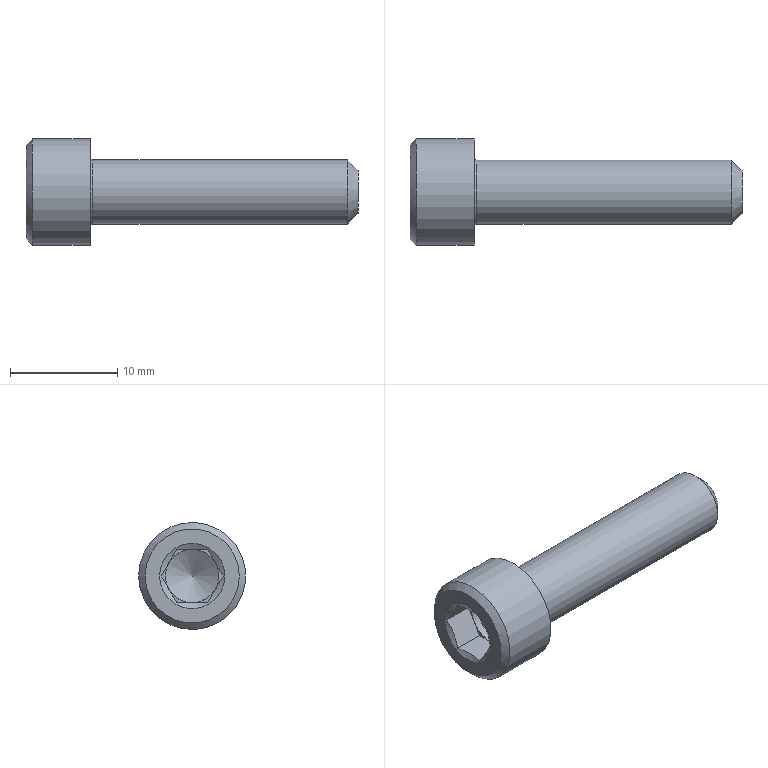Part | STEP file | Винт М6-6gx25 ГОСТ 11738-84 | 1 solid | 23 faces | box 31 x 10 x 10 mm | volume 1075 mm3 | plane 15 | cone 4 | cylinder 3 | torus 1 | commonest cylinder face diameters 5 x1 6 x1 10 x1
STEP:
#1=CARTESIAN_POINT('',(-6.,4.4,0.));
#2=VERTEX_POINT('',#1);
#3=CARTESIAN_POINT('',(-6.,0.,0.));
#4=DIRECTION('',(1.,0.,0.));
#5=DIRECTION('',(0.,1.,0.));
#6=AXIS2_PLACEMENT_3D('',#3,#4,#5);
#7=CIRCLE('',#6,4.4);
#8=EDGE_CURVE('',#2,#2,#7,.T.);
#9=ORIENTED_EDGE('',*,*,#8,.F.);
#10=EDGE_LOOP('',(#9));
#11=FACE_BOUND('',#10,.T.);
#12=CARTESIAN_POINT('',(-6.,3.05,0.));
#13=VERTEX_POINT('',#12);
#14=CARTESIAN_POINT('',(-6.,0.,0.));
#15=DIRECTION('',(1.,0.,0.));
#16=DIRECTION('',(0.,1.,0.));
#17=AXIS2_PLACEMENT_3D('',#14,#15,#16);
#18=CIRCLE('',#17,3.05);
#19=EDGE_CURVE('',#13,#13,#18,.T.);
#20=ORIENTED_EDGE('',*,*,#19,.T.);
#21=EDGE_LOOP('',(#20));
#22=FACE_BOUND('',#21,.T.);
#23=CARTESIAN_POINT('',(-6.,0.,0.));
#24=DIRECTION('',(-1.,0.,0.));
#25=DIRECTION('',(0.,1.,0.));
#26=AXIS2_PLACEMENT_3D('',#23,#24,#25);
#27=PLANE('',#26);
#28=ADVANCED_FACE('',(#11,#22),#27,.T.);
#29=CARTESIAN_POINT('',(-5.906,1.443,-2.5));
#30=VERTEX_POINT('',#29);
#31=CARTESIAN_POINT('',(-5.906,-1.443,-2.5));
#32=VERTEX_POINT('',#31);
#33=CARTESIAN_POINT('',(-5.906,1.443,-2.5));
#34=CARTESIAN_POINT('',(-5.9,1.424,-2.5));
#35=CARTESIAN_POINT('',(-5.89,1.389,-2.5));
#36=CARTESIAN_POINT('',(-5.88,1.351,-2.5));
#37=CARTESIAN_POINT('',(-5.867,1.304,-2.5));
#38=CARTESIAN_POINT('',(-5.848,1.232,-2.5));
#39=CARTESIAN_POINT('',(-5.827,1.146,-2.5));
#40=CARTESIAN_POINT('',(-5.803,1.043,-2.5));
#41=CARTESIAN_POINT('',(-5.774,0.909,-2.5));
#42=CARTESIAN_POINT('',(-5.75,0.7773,-2.5));
#43=CARTESIAN_POINT('',(-5.728,0.6356,-2.5));
#44=CARTESIAN_POINT('',(-5.711,0.5115,-2.5));
#45=CARTESIAN_POINT('',(-5.699,0.3892,-2.5));
#46=CARTESIAN_POINT('',(-5.692,0.2947,-2.5));
#47=CARTESIAN_POINT('',(-5.688,0.2222,-2.5));
#48=CARTESIAN_POINT('',(-5.684,0.1323,-2.5));
#49=CARTESIAN_POINT('',(-5.683,0.05578,-2.5));
#50=CARTESIAN_POINT('',(-5.682,-0.001577,-2.5));
#51=CARTESIAN_POINT('',(-5.683,-0.03169,-2.5));
#52=CARTESIAN_POINT('',(-5.683,-0.0738,-2.5));
#53=CARTESIAN_POINT('',(-5.684,-0.1276,-2.5));
#54=CARTESIAN_POINT('',(-5.687,-0.2055,-2.5));
#55=CARTESIAN_POINT('',(-5.692,-0.2839,-2.5));
#56=CARTESIAN_POINT('',(-5.696,-0.3444,-2.5));
#57=CARTESIAN_POINT('',(-5.7,-0.3959,-2.5));
#58=CARTESIAN_POINT('',(-5.705,-0.4472,-2.5));
#59=CARTESIAN_POINT('',(-5.713,-0.5148,-2.5));
#60=CARTESIAN_POINT('',(-5.722,-0.5907,-2.5));
#61=CARTESIAN_POINT('',(-5.73,-0.6507,-2.5));
#62=CARTESIAN_POINT('',(-5.738,-0.7005,-2.5));
#63=CARTESIAN_POINT('',(-5.746,-0.7498,-2.5));
#64=CARTESIAN_POINT('',(-5.757,-0.8136,-2.5));
#65=CARTESIAN_POINT('',(-5.77,-0.8864,-2.5));
#66=CARTESIAN_POINT('',(-5.785,-0.9583,-2.5));
#67=CARTESIAN_POINT('',(-5.8,-1.03,-2.5));
#68=CARTESIAN_POINT('',(-5.812,-1.084,-2.5));
#69=CARTESIAN_POINT('',(-5.823,-1.131,-2.5));
#70=CARTESIAN_POINT('',(-5.834,-1.177,-2.5));
#71=CARTESIAN_POINT('',(-5.85,-1.239,-2.5));
#72=CARTESIAN_POINT('',(-5.868,-1.307,-2.5));
#73=CARTESIAN_POINT('',(-5.882,-1.361,-2.5));
#74=CARTESIAN_POINT('',(-5.895,-1.406,-2.5));
#75=CARTESIAN_POINT('',(-5.902,-1.429,-2.5));
#76=CARTESIAN_POINT('',(-5.906,-1.443,-2.5));
#77=B_SPLINE_CURVE_WITH_KNOTS('',3,(#33,#34,#35,#36,#37,#38,#39,#40,#41,#42,#43,#44,#45,#46,#47,#48,#49,#50,#51,#52,#53,#54,#55,#56,#57,#58,#59,#60,#61,#62,#63,#64,#65,#66,#67,#68,#69,#70,#71,#72,#73,#74,#75,#76),.UNSPECIFIED.,.F.,.F.,(4,1,1,1,1,1,1,1,1,1,1,1,1,1,1,1,1,1,1,1,1,1,1,1,1,1,1,1,1,1,1,1,1,1,1,1,1,1,1,1,1,4),(0.,0.02097,0.03685,0.04095,0.07015,0.1134,0.1316,0.1778,0.2541,0.2686,0.3246,0.3823,0.3943,0.4217,0.4566,0.4863,0.5,0.5153,0.5171,0.5431,0.5703,0.5969,0.6234,0.6325,0.6498,0.6761,0.7022,0.7281,0.7381,0.7538,0.7792,0.8044,0.8294,0.8543,0.8789,0.8866,0.9033,0.9276,0.9518,0.9759,0.9843,1.),.UNSPECIFIED.);
#78=EDGE_CURVE('',#30,#32,#77,.T.);
#79=ORIENTED_EDGE('',*,*,#78,.T.);
#80=CARTESIAN_POINT('',(-3.,-1.443,-2.5));
#81=VERTEX_POINT('',#80);
#82=CARTESIAN_POINT('',(-3.,-1.443,-2.5));
#83=DIRECTION('',(-1.,0.,0.));
#84=VECTOR('',#83,1.);
#85=LINE('',#82,#84);
#86=EDGE_CURVE('',#81,#32,#85,.T.);
#87=ORIENTED_EDGE('',*,*,#86,.F.);
#88=CARTESIAN_POINT('',(-3.,0.,-2.5));
#89=VERTEX_POINT('',#88);
#90=CARTESIAN_POINT('',(-3.,0.,-2.5));
#91=DIRECTION('',(0.,-1.,0.));
#92=VECTOR('',#91,1.);
#93=LINE('',#90,#92);
#94=EDGE_CURVE('',#89,#81,#93,.T.);
#95=ORIENTED_EDGE('',*,*,#94,.F.);
#96=CARTESIAN_POINT('',(-3.,1.443,-2.5));
#97=VERTEX_POINT('',#96);
#98=CARTESIAN_POINT('',(-3.,1.443,-2.5));
#99=DIRECTION('',(0.,-1.,0.));
#100=VECTOR('',#99,1.);
#101=LINE('',#98,#100);
#102=EDGE_CURVE('',#97,#89,#101,.T.);
#103=ORIENTED_EDGE('',*,*,#102,.F.);
#104=CARTESIAN_POINT('',(-3.,1.443,-2.5));
#105=DIRECTION('',(-1.,0.,0.));
#106=VECTOR('',#105,1.);
#107=LINE('',#104,#106);
#108=EDGE_CURVE('',#97,#30,#107,.T.);
#109=ORIENTED_EDGE('',*,*,#108,.T.);
#110=EDGE_LOOP('',(#79,#87,#95,#103,#109));
#111=FACE_BOUND('',#110,.T.);
#112=CARTESIAN_POINT('',(-3.,1.443,-2.5));
#113=DIRECTION('',(0.,0.,-1.));
#114=DIRECTION('',(0.,-1.,0.));
#115=AXIS2_PLACEMENT_3D('',#112,#113,#114);
#116=PLANE('',#115);
#117=ADVANCED_FACE('',(#111),#116,.F.);
#118=CARTESIAN_POINT('',(-5.906,-2.887,0.));
#119=VERTEX_POINT('',#118);
#120=CARTESIAN_POINT('',(-5.906,-1.443,-2.5));
#121=CARTESIAN_POINT('',(-5.9,-1.453,-2.483));
#122=CARTESIAN_POINT('',(-5.889,-1.472,-2.45));
#123=CARTESIAN_POINT('',(-5.871,-1.505,-2.392));
#124=CARTESIAN_POINT('',(-5.848,-1.549,-2.317));
#125=CARTESIAN_POINT('',(-5.816,-1.614,-2.204));
#126=CARTESIAN_POINT('',(-5.777,-1.702,-2.052));
#127=CARTESIAN_POINT('',(-5.74,-1.803,-1.877));
#128=CARTESIAN_POINT('',(-5.713,-1.902,-1.705));
#129=CARTESIAN_POINT('',(-5.697,-1.984,-1.564));
#130=CARTESIAN_POINT('',(-5.688,-2.048,-1.453));
#131=CARTESIAN_POINT('',(-5.684,-2.099,-1.365));
#132=CARTESIAN_POINT('',(-5.683,-2.137,-1.298));
#133=CARTESIAN_POINT('',(-5.682,-2.166,-1.249));
#134=CARTESIAN_POINT('',(-5.683,-2.194,-1.201));
#135=CARTESIAN_POINT('',(-5.684,-2.228,-1.141));
#136=CARTESIAN_POINT('',(-5.687,-2.268,-1.072));
#137=CARTESIAN_POINT('',(-5.692,-2.307,-1.004));
#138=CARTESIAN_POINT('',(-5.697,-2.346,-0.9371));
#139=CARTESIAN_POINT('',(-5.704,-2.384,-0.8704));
#140=CARTESIAN_POINT('',(-5.713,-2.422,-0.8041));
#141=CARTESIAN_POINT('',(-5.722,-2.46,-0.7384));
#142=CARTESIAN_POINT('',(-5.733,-2.498,-0.6734));
#143=CARTESIAN_POINT('',(-5.744,-2.535,-0.609));
#144=CARTESIAN_POINT('',(-5.757,-2.572,-0.5454));
#145=CARTESIAN_POINT('',(-5.77,-2.608,-0.4824));
#146=CARTESIAN_POINT('',(-5.785,-2.644,-0.4201));
#147=CARTESIAN_POINT('',(-5.8,-2.68,-0.3584));
#148=CARTESIAN_POINT('',(-5.816,-2.715,-0.2974));
#149=CARTESIAN_POINT('',(-5.832,-2.75,-0.237));
#150=CARTESIAN_POINT('',(-5.85,-2.784,-0.1771));
#151=CARTESIAN_POINT('',(-5.868,-2.819,-0.1177));
#152=CARTESIAN_POINT('',(-5.886,-2.853,-0.05869));
#153=CARTESIAN_POINT('',(-5.899,-2.875,-0.01952));
#154=CARTESIAN_POINT('',(-5.906,-2.887,0.));
#155=B_SPLINE_CURVE_WITH_KNOTS('',3,(#120,#121,#122,#123,#124,#125,#126,#127,#128,#129,#130,#131,#132,#133,#134,#135,#136,#137,#138,#139,#140,#141,#142,#143,#144,#145,#146,#147,#148,#149,#150,#151,#152,#153,#154),.UNSPECIFIED.,.F.,.F.,(4,1,1,1,1,1,1,1,1,1,1,1,1,1,1,1,1,1,1,1,1,1,1,1,1,1,1,1,1,1,1,1,4),(0.,0.02097,0.04095,0.07015,0.1134,0.1778,0.2541,0.3246,0.3823,0.4217,0.4566,0.4863,0.5,0.5153,0.5431,0.5703,0.5969,0.6234,0.6498,0.6761,0.7022,0.7281,0.7538,0.7792,0.8044,0.8294,0.8543,0.8789,0.9033,0.9276,0.9518,0.9759,1.),.UNSPECIFIED.);
#156=EDGE_CURVE('',#32,#119,#155,.T.);
#157=ORIENTED_EDGE('',*,*,#156,.T.);
#158=CARTESIAN_POINT('',(-3.,-2.887,0.));
#159=VERTEX_POINT('',#158);
#160=CARTESIAN_POINT('',(-3.,-2.887,0.));
#161=DIRECTION('',(-1.,0.,0.));
#162=VECTOR('',#161,1.);
#163=LINE('',#160,#162);
#164=EDGE_CURVE('',#159,#119,#163,.T.);
#165=ORIENTED_EDGE('',*,*,#164,.F.);
#166=CARTESIAN_POINT('',(-3.,-2.165,-1.25));
#167=VERTEX_POINT('',#166);
#168=CARTESIAN_POINT('',(-3.,-2.165,-1.25));
#169=DIRECTION('',(0.,-0.5,0.866));
#170=VECTOR('',#169,1.);
#171=LINE('',#168,#170);
#172=EDGE_CURVE('',#167,#159,#171,.T.);
#173=ORIENTED_EDGE('',*,*,#172,.F.);
#174=CARTESIAN_POINT('',(-3.,-1.443,-2.5));
#175=DIRECTION('',(0.,-0.5,0.866));
#176=VECTOR('',#175,1.);
#177=LINE('',#174,#176);
#178=EDGE_CURVE('',#81,#167,#177,.T.);
#179=ORIENTED_EDGE('',*,*,#178,.F.);
#180=ORIENTED_EDGE('',*,*,#86,.T.);
#181=EDGE_LOOP('',(#157,#165,#173,#179,#180));
#182=FACE_BOUND('',#181,.T.);
#183=CARTESIAN_POINT('',(-3.,-1.443,-2.5));
#184=DIRECTION('',(0.,-0.866,-0.5));
#185=DIRECTION('',(0.,-0.5,0.866));
#186=AXIS2_PLACEMENT_3D('',#183,#184,#185);
#187=PLANE('',#186);
#188=ADVANCED_FACE('',(#182),#187,.F.);
#189=CARTESIAN_POINT('',(-5.906,-1.443,2.5));
#190=VERTEX_POINT('',#189);
#191=CARTESIAN_POINT('',(-5.906,-2.887,0.));
#192=CARTESIAN_POINT('',(-5.9,-2.877,0.01704));
#193=CARTESIAN_POINT('',(-5.889,-2.858,0.05036));
#194=CARTESIAN_POINT('',(-5.871,-2.825,0.1076));
#195=CARTESIAN_POINT('',(-5.848,-2.781,0.1832));
#196=CARTESIAN_POINT('',(-5.816,-2.716,0.2956));
#197=CARTESIAN_POINT('',(-5.777,-2.628,0.4476));
#198=CARTESIAN_POINT('',(-5.74,-2.527,0.6235));
#199=CARTESIAN_POINT('',(-5.713,-2.428,0.7948));
#200=CARTESIAN_POINT('',(-5.697,-2.346,0.936));
#201=CARTESIAN_POINT('',(-5.688,-2.282,1.047));
#202=CARTESIAN_POINT('',(-5.684,-2.231,1.135));
#203=CARTESIAN_POINT('',(-5.683,-2.193,1.202));
#204=CARTESIAN_POINT('',(-5.682,-2.164,1.251));
#205=CARTESIAN_POINT('',(-5.683,-2.137,1.299));
#206=CARTESIAN_POINT('',(-5.684,-2.102,1.359));
#207=CARTESIAN_POINT('',(-5.687,-2.062,1.428));
#208=CARTESIAN_POINT('',(-5.692,-2.023,1.496));
#209=CARTESIAN_POINT('',(-5.697,-1.984,1.563));
#210=CARTESIAN_POINT('',(-5.704,-1.946,1.63));
#211=CARTESIAN_POINT('',(-5.713,-1.908,1.696));
#212=CARTESIAN_POINT('',(-5.722,-1.87,1.762));
#213=CARTESIAN_POINT('',(-5.733,-1.832,1.827));
#214=CARTESIAN_POINT('',(-5.744,-1.795,1.891));
#215=CARTESIAN_POINT('',(-5.757,-1.758,1.955));
#216=CARTESIAN_POINT('',(-5.77,-1.722,2.018));
#217=CARTESIAN_POINT('',(-5.785,-1.686,2.08));
#218=CARTESIAN_POINT('',(-5.8,-1.65,2.142));
#219=CARTESIAN_POINT('',(-5.816,-1.615,2.203));
#220=CARTESIAN_POINT('',(-5.832,-1.58,2.263));
#221=CARTESIAN_POINT('',(-5.85,-1.546,2.323));
#222=CARTESIAN_POINT('',(-5.868,-1.511,2.382));
#223=CARTESIAN_POINT('',(-5.886,-1.477,2.441));
#224=CARTESIAN_POINT('',(-5.899,-1.455,2.48));
#225=CARTESIAN_POINT('',(-5.906,-1.443,2.5));
#226=B_SPLINE_CURVE_WITH_KNOTS('',3,(#191,#192,#193,#194,#195,#196,#197,#198,#199,#200,#201,#202,#203,#204,#205,#206,#207,#208,#209,#210,#211,#212,#213,#214,#215,#216,#217,#218,#219,#220,#221,#222,#223,#224,#225),.UNSPECIFIED.,.F.,.F.,(4,1,1,1,1,1,1,1,1,1,1,1,1,1,1,1,1,1,1,1,1,1,1,1,1,1,1,1,1,1,1,1,4),(0.,0.02097,0.04095,0.07015,0.1134,0.1778,0.2541,0.3246,0.3823,0.4217,0.4566,0.4863,0.5,0.5153,0.5431,0.5703,0.5969,0.6234,0.6498,0.6761,0.7022,0.7281,0.7538,0.7792,0.8044,0.8294,0.8543,0.8789,0.9033,0.9276,0.9518,0.9759,1.),.UNSPECIFIED.);
#227=EDGE_CURVE('',#119,#190,#226,.T.);
#228=ORIENTED_EDGE('',*,*,#227,.T.);
#229=CARTESIAN_POINT('',(-3.,-1.443,2.5));
#230=VERTEX_POINT('',#229);
#231=CARTESIAN_POINT('',(-3.,-1.443,2.5));
#232=DIRECTION('',(-1.,0.,0.));
#233=VECTOR('',#232,1.);
#234=LINE('',#231,#233);
#235=EDGE_CURVE('',#230,#190,#234,.T.);
#236=ORIENTED_EDGE('',*,*,#235,.F.);
#237=CARTESIAN_POINT('',(-3.,-2.165,1.25));
#238=VERTEX_POINT('',#237);
#239=CARTESIAN_POINT('',(-3.,-2.165,1.25));
#240=DIRECTION('',(0.,0.5,0.866));
#241=VECTOR('',#240,1.);
#242=LINE('',#239,#241);
#243=EDGE_CURVE('',#238,#230,#242,.T.);
#244=ORIENTED_EDGE('',*,*,#243,.F.);
#245=CARTESIAN_POINT('',(-3.,-2.887,0.));
#246=DIRECTION('',(0.,0.5,0.866));
#247=VECTOR('',#246,1.);
#248=LINE('',#245,#247);
#249=EDGE_CURVE('',#159,#238,#248,.T.);
#250=ORIENTED_EDGE('',*,*,#249,.F.);
#251=ORIENTED_EDGE('',*,*,#164,.T.);
#252=EDGE_LOOP('',(#228,#236,#244,#250,#251));
#253=FACE_BOUND('',#252,.T.);
#254=CARTESIAN_POINT('',(-3.,-2.887,0.));
#255=DIRECTION('',(0.,-0.866,0.5));
#256=DIRECTION('',(0.,0.5,0.866));
#257=AXIS2_PLACEMENT_3D('',#254,#255,#256);
#258=PLANE('',#257);
#259=ADVANCED_FACE('',(#253),#258,.F.);
#260=CARTESIAN_POINT('',(-5.906,1.443,2.5));
#261=VERTEX_POINT('',#260);
#262=CARTESIAN_POINT('',(-5.906,-1.443,2.5));
#263=CARTESIAN_POINT('',(-5.9,-1.424,2.5));
#264=CARTESIAN_POINT('',(-5.89,-1.389,2.5));
#265=CARTESIAN_POINT('',(-5.88,-1.351,2.5));
#266=CARTESIAN_POINT('',(-5.867,-1.304,2.5));
#267=CARTESIAN_POINT('',(-5.848,-1.232,2.5));
#268=CARTESIAN_POINT('',(-5.827,-1.146,2.5));
#269=CARTESIAN_POINT('',(-5.803,-1.043,2.5));
#270=CARTESIAN_POINT('',(-5.774,-0.909,2.5));
#271=CARTESIAN_POINT('',(-5.75,-0.7773,2.5));
#272=CARTESIAN_POINT('',(-5.728,-0.6356,2.5));
#273=CARTESIAN_POINT('',(-5.711,-0.5115,2.5));
#274=CARTESIAN_POINT('',(-5.699,-0.3892,2.5));
#275=CARTESIAN_POINT('',(-5.692,-0.2947,2.5));
#276=CARTESIAN_POINT('',(-5.688,-0.2222,2.5));
#277=CARTESIAN_POINT('',(-5.684,-0.1323,2.5));
#278=CARTESIAN_POINT('',(-5.683,-0.05578,2.5));
#279=CARTESIAN_POINT('',(-5.682,0.001577,2.5));
#280=CARTESIAN_POINT('',(-5.683,0.03169,2.5));
#281=CARTESIAN_POINT('',(-5.683,0.0738,2.5));
#282=CARTESIAN_POINT('',(-5.684,0.1276,2.5));
#283=CARTESIAN_POINT('',(-5.687,0.2055,2.5));
#284=CARTESIAN_POINT('',(-5.692,0.2839,2.5));
#285=CARTESIAN_POINT('',(-5.696,0.3444,2.5));
#286=CARTESIAN_POINT('',(-5.7,0.3959,2.5));
#287=CARTESIAN_POINT('',(-5.705,0.4472,2.5));
#288=CARTESIAN_POINT('',(-5.713,0.5148,2.5));
#289=CARTESIAN_POINT('',(-5.722,0.5907,2.5));
#290=CARTESIAN_POINT('',(-5.73,0.6507,2.5));
#291=CARTESIAN_POINT('',(-5.738,0.7005,2.5));
#292=CARTESIAN_POINT('',(-5.746,0.7498,2.5));
#293=CARTESIAN_POINT('',(-5.757,0.8136,2.5));
#294=CARTESIAN_POINT('',(-5.77,0.8864,2.5));
#295=CARTESIAN_POINT('',(-5.785,0.9583,2.5));
#296=CARTESIAN_POINT('',(-5.8,1.03,2.5));
#297=CARTESIAN_POINT('',(-5.812,1.084,2.5));
#298=CARTESIAN_POINT('',(-5.823,1.131,2.5));
#299=CARTESIAN_POINT('',(-5.834,1.177,2.5));
#300=CARTESIAN_POINT('',(-5.85,1.239,2.5));
#301=CARTESIAN_POINT('',(-5.868,1.307,2.5));
#302=CARTESIAN_POINT('',(-5.882,1.361,2.5));
#303=CARTESIAN_POINT('',(-5.895,1.406,2.5));
#304=CARTESIAN_POINT('',(-5.902,1.429,2.5));
#305=CARTESIAN_POINT('',(-5.906,1.443,2.5));
#306=B_SPLINE_CURVE_WITH_KNOTS('',3,(#262,#263,#264,#265,#266,#267,#268,#269,#270,#271,#272,#273,#274,#275,#276,#277,#278,#279,#280,#281,#282,#283,#284,#285,#286,#287,#288,#289,#290,#291,#292,#293,#294,#295,#296,#297,#298,#299,#300,#301,#302,#303,#304,#305),.UNSPECIFIED.,.F.,.F.,(4,1,1,1,1,1,1,1,1,1,1,1,1,1,1,1,1,1,1,1,1,1,1,1,1,1,1,1,1,1,1,1,1,1,1,1,1,1,1,1,1,4),(0.,0.02097,0.03685,0.04095,0.07015,0.1134,0.1316,0.1778,0.2541,0.2686,0.3246,0.3823,0.3943,0.4217,0.4566,0.4863,0.5,0.5153,0.5171,0.5431,0.5703,0.5969,0.6234,0.6325,0.6498,0.6761,0.7022,0.7281,0.7381,0.7538,0.7792,0.8044,0.8294,0.8543,0.8789,0.8866,0.9033,0.9276,0.9518,0.9759,0.9843,1.),.UNSPECIFIED.);
#307=EDGE_CURVE('',#190,#261,#306,.T.);
#308=ORIENTED_EDGE('',*,*,#307,.T.);
#309=CARTESIAN_POINT('',(-3.,1.443,2.5));
#310=VERTEX_POINT('',#309);
#311=CARTESIAN_POINT('',(-3.,1.443,2.5));
#312=DIRECTION('',(-1.,0.,0.));
#313=VECTOR('',#312,1.);
#314=LINE('',#311,#313);
#315=EDGE_CURVE('',#310,#261,#314,.T.);
#316=ORIENTED_EDGE('',*,*,#315,.F.);
#317=CARTESIAN_POINT('',(-3.,0.,2.5));
#318=VERTEX_POINT('',#317);
#319=CARTESIAN_POINT('',(-3.,0.,2.5));
#320=DIRECTION('',(0.,1.,0.));
#321=VECTOR('',#320,1.);
#322=LINE('',#319,#321);
#323=EDGE_CURVE('',#318,#310,#322,.T.);
#324=ORIENTED_EDGE('',*,*,#323,.F.);
#325=CARTESIAN_POINT('',(-3.,-1.443,2.5));
#326=DIRECTION('',(0.,1.,0.));
#327=VECTOR('',#326,1.);
#328=LINE('',#325,#327);
#329=EDGE_CURVE('',#230,#318,#328,.T.);
#330=ORIENTED_EDGE('',*,*,#329,.F.);
#331=ORIENTED_EDGE('',*,*,#235,.T.);
#332=EDGE_LOOP('',(#308,#316,#324,#330,#331));
#333=FACE_BOUND('',#332,.T.);
#334=CARTESIAN_POINT('',(-3.,-1.443,2.5));
#335=DIRECTION('',(0.,0.,1.));
#336=DIRECTION('',(0.,1.,0.));
#337=AXIS2_PLACEMENT_3D('',#334,#335,#336);
#338=PLANE('',#337);
#339=ADVANCED_FACE('',(#333),#338,.F.);
#340=CARTESIAN_POINT('',(-5.906,2.887,0.));
#341=VERTEX_POINT('',#340);
#342=CARTESIAN_POINT('',(-5.906,2.887,0.));
#343=CARTESIAN_POINT('',(-5.9,2.877,-0.01704));
#344=CARTESIAN_POINT('',(-5.889,2.858,-0.05036));
#345=CARTESIAN_POINT('',(-5.871,2.825,-0.1076));
#346=CARTESIAN_POINT('',(-5.848,2.781,-0.1832));
#347=CARTESIAN_POINT('',(-5.816,2.716,-0.2956));
#348=CARTESIAN_POINT('',(-5.777,2.628,-0.4476));
#349=CARTESIAN_POINT('',(-5.74,2.527,-0.6235));
#350=CARTESIAN_POINT('',(-5.713,2.428,-0.7948));
#351=CARTESIAN_POINT('',(-5.697,2.346,-0.936));
#352=CARTESIAN_POINT('',(-5.688,2.282,-1.047));
#353=CARTESIAN_POINT('',(-5.684,2.231,-1.135));
#354=CARTESIAN_POINT('',(-5.683,2.193,-1.202));
#355=CARTESIAN_POINT('',(-5.682,2.164,-1.251));
#356=CARTESIAN_POINT('',(-5.683,2.137,-1.299));
#357=CARTESIAN_POINT('',(-5.684,2.102,-1.359));
#358=CARTESIAN_POINT('',(-5.687,2.062,-1.428));
#359=CARTESIAN_POINT('',(-5.692,2.023,-1.496));
#360=CARTESIAN_POINT('',(-5.697,1.984,-1.563));
#361=CARTESIAN_POINT('',(-5.704,1.946,-1.63));
#362=CARTESIAN_POINT('',(-5.713,1.908,-1.696));
#363=CARTESIAN_POINT('',(-5.722,1.87,-1.762));
#364=CARTESIAN_POINT('',(-5.733,1.832,-1.827));
#365=CARTESIAN_POINT('',(-5.744,1.795,-1.891));
#366=CARTESIAN_POINT('',(-5.757,1.758,-1.955));
#367=CARTESIAN_POINT('',(-5.77,1.722,-2.018));
#368=CARTESIAN_POINT('',(-5.785,1.686,-2.08));
#369=CARTESIAN_POINT('',(-5.8,1.65,-2.142));
#370=CARTESIAN_POINT('',(-5.816,1.615,-2.203));
#371=CARTESIAN_POINT('',(-5.832,1.58,-2.263));
#372=CARTESIAN_POINT('',(-5.85,1.546,-2.323));
#373=CARTESIAN_POINT('',(-5.868,1.511,-2.382));
#374=CARTESIAN_POINT('',(-5.886,1.477,-2.441));
#375=CARTESIAN_POINT('',(-5.899,1.455,-2.48));
#376=CARTESIAN_POINT('',(-5.906,1.443,-2.5));
#377=B_SPLINE_CURVE_WITH_KNOTS('',3,(#342,#343,#344,#345,#346,#347,#348,#349,#350,#351,#352,#353,#354,#355,#356,#357,#358,#359,#360,#361,#362,#363,#364,#365,#366,#367,#368,#369,#370,#371,#372,#373,#374,#375,#376),.UNSPECIFIED.,.F.,.F.,(4,1,1,1,1,1,1,1,1,1,1,1,1,1,1,1,1,1,1,1,1,1,1,1,1,1,1,1,1,1,1,1,4),(0.,0.02097,0.04095,0.07015,0.1134,0.1778,0.2541,0.3246,0.3823,0.4217,0.4566,0.4863,0.5,0.5153,0.5431,0.5703,0.5969,0.6234,0.6498,0.6761,0.7022,0.7281,0.7538,0.7792,0.8044,0.8294,0.8543,0.8789,0.9033,0.9276,0.9518,0.9759,1.),.UNSPECIFIED.);
#378=EDGE_CURVE('',#341,#30,#377,.T.);
#379=ORIENTED_EDGE('',*,*,#378,.T.);
#380=ORIENTED_EDGE('',*,*,#108,.F.);
#381=CARTESIAN_POINT('',(-3.,2.165,-1.25));
#382=VERTEX_POINT('',#381);
#383=CARTESIAN_POINT('',(-3.,2.165,-1.25));
#384=DIRECTION('',(0.,-0.5,-0.866));
#385=VECTOR('',#384,1.);
#386=LINE('',#383,#385);
#387=EDGE_CURVE('',#382,#97,#386,.T.);
#388=ORIENTED_EDGE('',*,*,#387,.F.);
#389=CARTESIAN_POINT('',(-3.,2.887,0.));
#390=VERTEX_POINT('',#389);
#391=CARTESIAN_POINT('',(-3.,2.887,0.));
#392=DIRECTION('',(0.,-0.5,-0.866));
#393=VECTOR('',#392,1.);
#394=LINE('',#391,#393);
#395=EDGE_CURVE('',#390,#382,#394,.T.);
#396=ORIENTED_EDGE('',*,*,#395,.F.);
#397=CARTESIAN_POINT('',(-3.,2.887,0.));
#398=DIRECTION('',(-1.,0.,0.));
#399=VECTOR('',#398,1.);
#400=LINE('',#397,#399);
#401=EDGE_CURVE('',#390,#341,#400,.T.);
#402=ORIENTED_EDGE('',*,*,#401,.T.);
#403=EDGE_LOOP('',(#379,#380,#388,#396,#402));
#404=FACE_BOUND('',#403,.T.);
#405=CARTESIAN_POINT('',(-3.,2.887,0.));
#406=DIRECTION('',(0.,0.866,-0.5));
#407=DIRECTION('',(0.,-0.5,-0.866));
#408=AXIS2_PLACEMENT_3D('',#405,#406,#407);
#409=PLANE('',#408);
#410=ADVANCED_FACE('',(#404),#409,.F.);
#411=CARTESIAN_POINT('',(-5.906,1.443,2.5));
#412=CARTESIAN_POINT('',(-5.9,1.453,2.483));
#413=CARTESIAN_POINT('',(-5.889,1.472,2.45));
#414=CARTESIAN_POINT('',(-5.871,1.505,2.392));
#415=CARTESIAN_POINT('',(-5.848,1.549,2.317));
#416=CARTESIAN_POINT('',(-5.816,1.614,2.204));
#417=CARTESIAN_POINT('',(-5.777,1.702,2.052));
#418=CARTESIAN_POINT('',(-5.74,1.803,1.877));
#419=CARTESIAN_POINT('',(-5.713,1.902,1.705));
#420=CARTESIAN_POINT('',(-5.697,1.984,1.564));
#421=CARTESIAN_POINT('',(-5.688,2.048,1.453));
#422=CARTESIAN_POINT('',(-5.684,2.099,1.365));
#423=CARTESIAN_POINT('',(-5.683,2.137,1.298));
#424=CARTESIAN_POINT('',(-5.682,2.166,1.249));
#425=CARTESIAN_POINT('',(-5.683,2.194,1.201));
#426=CARTESIAN_POINT('',(-5.684,2.228,1.141));
#427=CARTESIAN_POINT('',(-5.687,2.268,1.072));
#428=CARTESIAN_POINT('',(-5.692,2.307,1.004));
#429=CARTESIAN_POINT('',(-5.697,2.346,0.9371));
#430=CARTESIAN_POINT('',(-5.704,2.384,0.8704));
#431=CARTESIAN_POINT('',(-5.713,2.422,0.8041));
#432=CARTESIAN_POINT('',(-5.722,2.46,0.7384));
#433=CARTESIAN_POINT('',(-5.733,2.498,0.6734));
#434=CARTESIAN_POINT('',(-5.744,2.535,0.609));
#435=CARTESIAN_POINT('',(-5.757,2.572,0.5454));
#436=CARTESIAN_POINT('',(-5.77,2.608,0.4824));
#437=CARTESIAN_POINT('',(-5.785,2.644,0.4201));
#438=CARTESIAN_POINT('',(-5.8,2.68,0.3584));
#439=CARTESIAN_POINT('',(-5.816,2.715,0.2974));
#440=CARTESIAN_POINT('',(-5.832,2.75,0.237));
#441=CARTESIAN_POINT('',(-5.85,2.784,0.1771));
#442=CARTESIAN_POINT('',(-5.868,2.819,0.1177));
#443=CARTESIAN_POINT('',(-5.886,2.853,0.05869));
#444=CARTESIAN_POINT('',(-5.899,2.875,0.01952));
#445=CARTESIAN_POINT('',(-5.906,2.887,0.));
#446=B_SPLINE_CURVE_WITH_KNOTS('',3,(#411,#412,#413,#414,#415,#416,#417,#418,#419,#420,#421,#422,#423,#424,#425,#426,#427,#428,#429,#430,#431,#432,#433,#434,#435,#436,#437,#438,#439,#440,#441,#442,#443,#444,#445),.UNSPECIFIED.,.F.,.F.,(4,1,1,1,1,1,1,1,1,1,1,1,1,1,1,1,1,1,1,1,1,1,1,1,1,1,1,1,1,1,1,1,4),(0.,0.02097,0.04095,0.07015,0.1134,0.1778,0.2541,0.3246,0.3823,0.4217,0.4566,0.4863,0.5,0.5153,0.5431,0.5703,0.5969,0.6234,0.6498,0.6761,0.7022,0.7281,0.7538,0.7792,0.8044,0.8294,0.8543,0.8789,0.9033,0.9276,0.9518,0.9759,1.),.UNSPECIFIED.);
#447=EDGE_CURVE('',#261,#341,#446,.T.);
#448=ORIENTED_EDGE('',*,*,#447,.T.);
#449=ORIENTED_EDGE('',*,*,#401,.F.);
#450=CARTESIAN_POINT('',(-3.,2.165,1.25));
#451=VERTEX_POINT('',#450);
#452=CARTESIAN_POINT('',(-3.,2.165,1.25));
#453=DIRECTION('',(0.,0.5,-0.866));
#454=VECTOR('',#453,1.);
#455=LINE('',#452,#454);
#456=EDGE_CURVE('',#451,#390,#455,.T.);
#457=ORIENTED_EDGE('',*,*,#456,.F.);
#458=CARTESIAN_POINT('',(-3.,1.443,2.5));
#459=DIRECTION('',(0.,0.5,-0.866));
#460=VECTOR('',#459,1.);
#461=LINE('',#458,#460);
#462=EDGE_CURVE('',#310,#451,#461,.T.);
#463=ORIENTED_EDGE('',*,*,#462,.F.);
#464=ORIENTED_EDGE('',*,*,#315,.T.);
#465=EDGE_LOOP('',(#448,#449,#457,#463,#464));
#466=FACE_BOUND('',#465,.T.);
#467=CARTESIAN_POINT('',(-3.,1.443,2.5));
#468=DIRECTION('',(0.,0.866,0.5));
#469=DIRECTION('',(0.,0.5,-0.866));
#470=AXIS2_PLACEMENT_3D('',#467,#468,#469);
#471=PLANE('',#470);
#472=ADVANCED_FACE('',(#466),#471,.F.);
#473=ORIENTED_EDGE('',*,*,#447,.F.);
#474=ORIENTED_EDGE('',*,*,#307,.F.);
#475=ORIENTED_EDGE('',*,*,#227,.F.);
#476=ORIENTED_EDGE('',*,*,#156,.F.);
#477=ORIENTED_EDGE('',*,*,#78,.F.);
#478=ORIENTED_EDGE('',*,*,#378,.F.);
#479=EDGE_LOOP('',(#473,#474,#475,#476,#477,#478));
#480=FACE_BOUND('',#479,.T.);
#481=ORIENTED_EDGE('',*,*,#19,.F.);
#482=EDGE_LOOP('',(#481));
#483=FACE_OUTER_BOUND('',#482,.T.);
#484=CARTESIAN_POINT('',(-5.841,0.,0.));
#485=DIRECTION('',(-1.,0.,0.));
#486=DIRECTION('',(0.,-1.,0.));
#487=AXIS2_PLACEMENT_3D('',#484,#485,#486);
#488=CONICAL_SURFACE('',#487,2.775,1.047);
#489=ADVANCED_FACE('',(#480,#483),#488,.F.);
#490=CARTESIAN_POINT('',(-5.4,5.,0.));
#491=VERTEX_POINT('',#490);
#492=CARTESIAN_POINT('',(-5.4,0.,0.));
#493=DIRECTION('',(1.,0.,0.));
#494=DIRECTION('',(0.,1.,0.));
#495=AXIS2_PLACEMENT_3D('',#492,#493,#494);
#496=CIRCLE('',#495,5.);
#497=EDGE_CURVE('',#491,#491,#496,.T.);
#498=ORIENTED_EDGE('',*,*,#497,.F.);
#499=EDGE_LOOP('',(#498));
#500=FACE_OUTER_BOUND('',#499,.T.);
#501=ORIENTED_EDGE('',*,*,#8,.T.);
#502=EDGE_LOOP('',(#501));
#503=FACE_OUTER_BOUND('',#502,.T.);
#504=CARTESIAN_POINT('',(-5.7,0.,0.));
#505=DIRECTION('',(1.,0.,0.));
#506=DIRECTION('',(0.,1.,0.));
#507=AXIS2_PLACEMENT_3D('',#504,#505,#506);
#508=CONICAL_SURFACE('',#507,4.7,0.7854);
#509=ADVANCED_FACE('',(#500,#503),#508,.T.);
#510=CARTESIAN_POINT('',(-3.,0.,0.));
#511=DIRECTION('',(1.,0.,0.));
#512=DIRECTION('',(0.,-0.866,-0.5));
#513=AXIS2_PLACEMENT_3D('',#510,#511,#512);
#514=CIRCLE('',#513,2.5);
#515=EDGE_CURVE('',#167,#89,#514,.T.);
#516=ORIENTED_EDGE('',*,*,#515,.T.);
#517=ORIENTED_EDGE('',*,*,#94,.T.);
#518=ORIENTED_EDGE('',*,*,#178,.T.);
#519=EDGE_LOOP('',(#516,#517,#518));
#520=FACE_BOUND('',#519,.T.);
#521=CARTESIAN_POINT('',(-3.,0.,0.));
#522=DIRECTION('',(-1.,0.,0.));
#523=DIRECTION('',(0.,0.,-1.));
#524=AXIS2_PLACEMENT_3D('',#521,#522,#523);
#525=PLANE('',#524);
#526=ADVANCED_FACE('',(#520),#525,.T.);
#527=CARTESIAN_POINT('',(-3.,0.,0.));
#528=DIRECTION('',(1.,0.,0.));
#529=DIRECTION('',(0.,0.,-1.));
#530=AXIS2_PLACEMENT_3D('',#527,#528,#529);
#531=CIRCLE('',#530,2.5);
#532=EDGE_CURVE('',#89,#382,#531,.T.);
#533=ORIENTED_EDGE('',*,*,#532,.T.);
#534=ORIENTED_EDGE('',*,*,#387,.T.);
#535=ORIENTED_EDGE('',*,*,#102,.T.);
#536=EDGE_LOOP('',(#533,#534,#535));
#537=FACE_BOUND('',#536,.T.);
#538=CARTESIAN_POINT('',(-3.,0.,0.));
#539=DIRECTION('',(-1.,0.,0.));
#540=DIRECTION('',(0.,0.,-1.));
#541=AXIS2_PLACEMENT_3D('',#538,#539,#540);
#542=PLANE('',#541);
#543=ADVANCED_FACE('',(#537),#542,.T.);
#544=CARTESIAN_POINT('',(-3.,0.,0.));
#545=DIRECTION('',(1.,0.,0.));
#546=DIRECTION('',(0.,-0.866,0.5));
#547=AXIS2_PLACEMENT_3D('',#544,#545,#546);
#548=CIRCLE('',#547,2.5);
#549=EDGE_CURVE('',#238,#167,#548,.T.);
#550=ORIENTED_EDGE('',*,*,#549,.T.);
#551=ORIENTED_EDGE('',*,*,#172,.T.);
#552=ORIENTED_EDGE('',*,*,#249,.T.);
#553=EDGE_LOOP('',(#550,#551,#552));
#554=FACE_BOUND('',#553,.T.);
#555=CARTESIAN_POINT('',(-3.,0.,0.));
#556=DIRECTION('',(-1.,0.,0.));
#557=DIRECTION('',(0.,0.,-1.));
#558=AXIS2_PLACEMENT_3D('',#555,#556,#557);
#559=PLANE('',#558);
#560=ADVANCED_FACE('',(#554),#559,.T.);
#561=CARTESIAN_POINT('',(-3.,0.,0.));
#562=DIRECTION('',(1.,0.,0.));
#563=DIRECTION('',(0.,0.,1.));
#564=AXIS2_PLACEMENT_3D('',#561,#562,#563);
#565=CIRCLE('',#564,2.5);
#566=EDGE_CURVE('',#318,#238,#565,.T.);
#567=ORIENTED_EDGE('',*,*,#566,.T.);
#568=ORIENTED_EDGE('',*,*,#243,.T.);
#569=ORIENTED_EDGE('',*,*,#329,.T.);
#570=EDGE_LOOP('',(#567,#568,#569));
#571=FACE_BOUND('',#570,.T.);
#572=CARTESIAN_POINT('',(-3.,0.,0.));
#573=DIRECTION('',(-1.,0.,0.));
#574=DIRECTION('',(0.,0.,-1.));
#575=AXIS2_PLACEMENT_3D('',#572,#573,#574);
#576=PLANE('',#575);
#577=ADVANCED_FACE('',(#571),#576,.T.);
#578=CARTESIAN_POINT('',(-3.,0.,0.));
#579=DIRECTION('',(1.,0.,0.));
#580=DIRECTION('',(0.,0.866,0.5));
#581=AXIS2_PLACEMENT_3D('',#578,#579,#580);
#582=CIRCLE('',#581,2.5);
#583=EDGE_CURVE('',#451,#318,#582,.T.);
#584=ORIENTED_EDGE('',*,*,#583,.T.);
#585=ORIENTED_EDGE('',*,*,#323,.T.);
#586=ORIENTED_EDGE('',*,*,#462,.T.);
#587=EDGE_LOOP('',(#584,#585,#586));
#588=FACE_BOUND('',#587,.T.);
#589=CARTESIAN_POINT('',(-3.,0.,0.));
#590=DIRECTION('',(-1.,0.,0.));
#591=DIRECTION('',(0.,0.,-1.));
#592=AXIS2_PLACEMENT_3D('',#589,#590,#591);
#593=PLANE('',#592);
#594=ADVANCED_FACE('',(#588),#593,.T.);
#595=CARTESIAN_POINT('',(-3.,2.5,0.));
#596=VERTEX_POINT('',#595);
#597=CARTESIAN_POINT('',(-3.,0.,0.));
#598=DIRECTION('',(1.,0.,0.));
#599=DIRECTION('',(0.,1.,0.));
#600=AXIS2_PLACEMENT_3D('',#597,#598,#599);
#601=CIRCLE('',#600,2.5);
#602=EDGE_CURVE('',#596,#451,#601,.T.);
#603=ORIENTED_EDGE('',*,*,#602,.T.);
#604=ORIENTED_EDGE('',*,*,#456,.T.);
#605=ORIENTED_EDGE('',*,*,#395,.T.);
#606=CARTESIAN_POINT('',(-3.,0.,0.));
#607=DIRECTION('',(1.,0.,0.));
#608=DIRECTION('',(0.,0.866,-0.5));
#609=AXIS2_PLACEMENT_3D('',#606,#607,#608);
#610=CIRCLE('',#609,2.5);
#611=EDGE_CURVE('',#382,#596,#610,.T.);
#612=ORIENTED_EDGE('',*,*,#611,.T.);
#613=EDGE_LOOP('',(#603,#604,#605,#612));
#614=FACE_BOUND('',#613,.T.);
#615=CARTESIAN_POINT('',(-3.,0.,0.));
#616=DIRECTION('',(-1.,0.,0.));
#617=DIRECTION('',(0.,0.,-1.));
#618=AXIS2_PLACEMENT_3D('',#615,#616,#617);
#619=PLANE('',#618);
#620=ADVANCED_FACE('',(#614),#619,.T.);
#621=CARTESIAN_POINT('',(0.,5.,0.));
#622=VERTEX_POINT('',#621);
#623=CARTESIAN_POINT('',(0.,0.,0.));
#624=DIRECTION('',(1.,0.,0.));
#625=DIRECTION('',(0.,1.,0.));
#626=AXIS2_PLACEMENT_3D('',#623,#624,#625);
#627=CIRCLE('',#626,5.);
#628=EDGE_CURVE('',#622,#622,#627,.T.);
#629=ORIENTED_EDGE('',*,*,#628,.F.);
#630=EDGE_LOOP('',(#629));
#631=FACE_OUTER_BOUND('',#630,.T.);
#632=ORIENTED_EDGE('',*,*,#497,.T.);
#633=EDGE_LOOP('',(#632));
#634=FACE_OUTER_BOUND('',#633,.T.);
#635=CARTESIAN_POINT('',(-6.,0.,0.));
#636=DIRECTION('',(1.,0.,0.));
#637=DIRECTION('',(0.,1.,0.));
#638=AXIS2_PLACEMENT_3D('',#635,#636,#637);
#639=CYLINDRICAL_SURFACE('',#638,5.);
#640=ADVANCED_FACE('',(#631,#634),#639,.T.);
#641=CARTESIAN_POINT('',(-2.3,2.5,0.));
#642=VERTEX_POINT('',#641);
#643=CARTESIAN_POINT('',(-2.3,0.,0.));
#644=DIRECTION('',(1.,0.,0.));
#645=DIRECTION('',(0.,1.,0.));
#646=AXIS2_PLACEMENT_3D('',#643,#644,#645);
#647=CIRCLE('',#646,2.5);
#648=EDGE_CURVE('',#642,#642,#647,.T.);
#649=ORIENTED_EDGE('',*,*,#648,.T.);
#650=EDGE_LOOP('',(#649));
#651=FACE_OUTER_BOUND('',#650,.T.);
#652=ORIENTED_EDGE('',*,*,#611,.F.);
#653=ORIENTED_EDGE('',*,*,#532,.F.);
#654=ORIENTED_EDGE('',*,*,#515,.F.);
#655=ORIENTED_EDGE('',*,*,#549,.F.);
#656=ORIENTED_EDGE('',*,*,#566,.F.);
#657=ORIENTED_EDGE('',*,*,#583,.F.);
#658=ORIENTED_EDGE('',*,*,#602,.F.);
#659=EDGE_LOOP('',(#652,#653,#654,#655,#656,#657,#658));
#660=FACE_BOUND('',#659,.T.);
#661=CARTESIAN_POINT('',(-6.,0.,0.));
#662=DIRECTION('',(1.,0.,0.));
#663=DIRECTION('',(0.,1.,0.));
#664=AXIS2_PLACEMENT_3D('',#661,#662,#663);
#665=CYLINDRICAL_SURFACE('',#664,2.5);
#666=ADVANCED_FACE('',(#651,#660),#665,.F.);
#667=ORIENTED_EDGE('',*,*,#628,.T.);
#668=EDGE_LOOP('',(#667));
#669=FACE_BOUND('',#668,.T.);
#670=CARTESIAN_POINT('',(0.,0.,-3.25));
#671=VERTEX_POINT('',#670);
#672=CARTESIAN_POINT('',(0.,0.,0.));
#673=DIRECTION('',(-1.,0.,0.));
#674=DIRECTION('',(0.,0.,-1.));
#675=AXIS2_PLACEMENT_3D('',#672,#673,#674);
#676=CIRCLE('',#675,3.25);
#677=EDGE_CURVE('',#671,#671,#676,.T.);
#678=ORIENTED_EDGE('',*,*,#677,.T.);
#679=EDGE_LOOP('',(#678));
#680=FACE_BOUND('',#679,.T.);
#681=CARTESIAN_POINT('',(0.,0.,0.));
#682=DIRECTION('',(1.,0.,0.));
#683=DIRECTION('',(0.,1.,0.));
#684=AXIS2_PLACEMENT_3D('',#681,#682,#683);
#685=PLANE('',#684);
#686=ADVANCED_FACE('',(#669,#680),#685,.T.);
#687=ORIENTED_EDGE('',*,*,#648,.F.);
#688=EDGE_LOOP('',(#687));
#689=FACE_OUTER_BOUND('',#688,.T.);
#690=CARTESIAN_POINT('',(-1.578,0.,0.));
#691=DIRECTION('',(-1.,0.,0.));
#692=DIRECTION('',(0.,-1.,0.));
#693=AXIS2_PLACEMENT_3D('',#690,#691,#692);
#694=CONICAL_SURFACE('',#693,1.25,1.047);
#695=ADVANCED_FACE('',(#689),#694,.F.);
#696=CARTESIAN_POINT('',(0.25,0.,-3.));
#697=VERTEX_POINT('',#696);
#698=CARTESIAN_POINT('',(0.25,0.,0.));
#699=DIRECTION('',(-1.,0.,0.));
#700=DIRECTION('',(0.,0.,-1.));
#701=AXIS2_PLACEMENT_3D('',#698,#699,#700);
#702=CIRCLE('',#701,3.);
#703=EDGE_CURVE('',#697,#697,#702,.T.);
#704=ORIENTED_EDGE('',*,*,#703,.T.);
#705=EDGE_LOOP('',(#704));
#706=FACE_OUTER_BOUND('',#705,.T.);
#707=ORIENTED_EDGE('',*,*,#677,.F.);
#708=EDGE_LOOP('',(#707));
#709=FACE_OUTER_BOUND('',#708,.T.);
#710=CARTESIAN_POINT('',(0.25,0.,0.));
#711=DIRECTION('',(-1.,0.,0.));
#712=DIRECTION('',(0.,0.,-1.));
#713=AXIS2_PLACEMENT_3D('',#710,#711,#712);
#714=TOROIDAL_SURFACE('',#713,3.25,0.25);
#715=ADVANCED_FACE('',(#706,#709),#714,.F.);
#716=CARTESIAN_POINT('',(24.,0.,-3.));
#717=VERTEX_POINT('',#716);
#718=CARTESIAN_POINT('',(24.,0.,0.));
#719=DIRECTION('',(-1.,0.,0.));
#720=DIRECTION('',(0.,0.,-1.));
#721=AXIS2_PLACEMENT_3D('',#718,#719,#720);
#722=CIRCLE('',#721,3.);
#723=EDGE_CURVE('',#717,#717,#722,.T.);
#724=ORIENTED_EDGE('',*,*,#723,.T.);
#725=EDGE_LOOP('',(#724));
#726=FACE_OUTER_BOUND('',#725,.T.);
#727=ORIENTED_EDGE('',*,*,#703,.F.);
#728=EDGE_LOOP('',(#727));
#729=FACE_OUTER_BOUND('',#728,.T.);
#730=CARTESIAN_POINT('',(25.,0.,0.));
#731=DIRECTION('',(-1.,0.,0.));
#732=DIRECTION('',(0.,0.,-1.));
#733=AXIS2_PLACEMENT_3D('',#730,#731,#732);
#734=CYLINDRICAL_SURFACE('',#733,3.);
#735=ADVANCED_FACE('',(#726,#729),#734,.T.);
#736=CARTESIAN_POINT('',(25.,0.,-2.));
#737=VERTEX_POINT('',#736);
#738=CARTESIAN_POINT('',(25.,0.,0.));
#739=DIRECTION('',(-1.,0.,0.));
#740=DIRECTION('',(0.,0.,-1.));
#741=AXIS2_PLACEMENT_3D('',#738,#739,#740);
#742=CIRCLE('',#741,2.);
#743=EDGE_CURVE('',#737,#737,#742,.T.);
#744=ORIENTED_EDGE('',*,*,#743,.F.);
#745=EDGE_LOOP('',(#744));
#746=FACE_BOUND('',#745,.T.);
#747=CARTESIAN_POINT('',(25.,0.,0.));
#748=DIRECTION('',(-1.,0.,0.));
#749=DIRECTION('',(0.,0.,-1.));
#750=AXIS2_PLACEMENT_3D('',#747,#748,#749);
#751=PLANE('',#750);
#752=ADVANCED_FACE('',(#746),#751,.F.);
#753=ORIENTED_EDGE('',*,*,#743,.T.);
#754=EDGE_LOOP('',(#753));
#755=FACE_OUTER_BOUND('',#754,.T.);
#756=ORIENTED_EDGE('',*,*,#723,.F.);
#757=EDGE_LOOP('',(#756));
#758=FACE_OUTER_BOUND('',#757,.T.);
#759=CARTESIAN_POINT('',(24.5,0.,0.));
#760=DIRECTION('',(-1.,0.,0.));
#761=DIRECTION('',(0.,0.,-1.));
#762=AXIS2_PLACEMENT_3D('',#759,#760,#761);
#763=CONICAL_SURFACE('',#762,2.5,0.7854);
#764=ADVANCED_FACE('',(#755,#758),#763,.T.);
#765=CLOSED_SHELL('',(#28,#117,#188,#259,#339,#410,#472,#489,#509,#526,#543,#560,#577,#594,#620,#640,#666,#686,#695,#715,#735,#752,#764));
#766=MANIFOLD_SOLID_BREP('',#765);
#767=(LENGTH_UNIT()NAMED_UNIT(*)SI_UNIT(.MILLI.,.METRE.));
#768=UNCERTAINTY_MEASURE_WITH_UNIT(LENGTH_MEASURE(0.00001),#767,'','');
#769=(NAMED_UNIT(*)PLANE_ANGLE_UNIT()SI_UNIT($,.RADIAN.));
#770=(NAMED_UNIT(*)SI_UNIT($,.STERADIAN.)SOLID_ANGLE_UNIT());
#771=(GEOMETRIC_REPRESENTATION_CONTEXT(3)GLOBAL_UNCERTAINTY_ASSIGNED_CONTEXT((#768))GLOBAL_UNIT_ASSIGNED_CONTEXT((#767,#769,#770))REPRESENTATION_CONTEXT('',''));
#772=ADVANCED_BREP_SHAPE_REPRESENTATION('',(#766),#771);